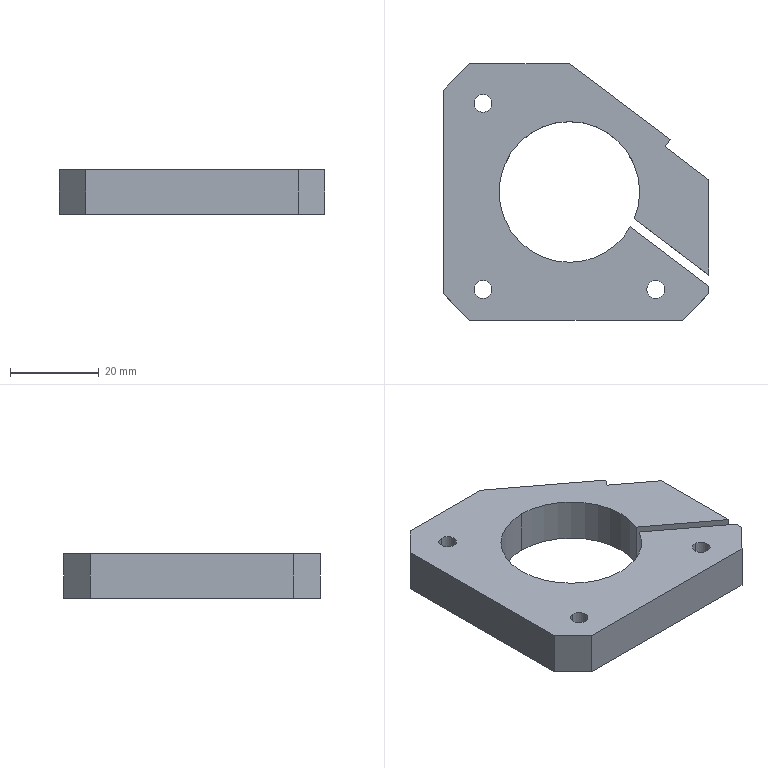Part | SolidWorks | features BaseBody 1 | 1 solid | 24 faces | box 60 x 58 x 10 mm | volume 21556 mm3 | plane 15 | cylinder 9 | commonest cylinder face diameters 4 x6 31.75 x3
STEP:
#1=CARTESIAN_POINT('',(17.98,-19.981,10.));
#2=VERTEX_POINT('',#1);
#3=CARTESIAN_POINT('',(17.98,-23.981,10.));
#4=VERTEX_POINT('',#3);
#5=CARTESIAN_POINT('',(17.98,-21.981,10.));
#6=DIRECTION('',(0.,0.,1.));
#7=DIRECTION('',(0.,1.,0.));
#8=AXIS2_PLACEMENT_3D('',#5,#6,#7);
#9=CIRCLE('',#8,2.);
#10=EDGE_CURVE('',#2,#4,#9,.T.);
#11=ORIENTED_EDGE('',*,*,#10,.T.);
#12=CARTESIAN_POINT('',(17.98,-23.981,0.));
#13=VERTEX_POINT('',#12);
#14=CARTESIAN_POINT('',(17.98,-23.981,10.));
#15=DIRECTION('',(0.,0.,-1.));
#16=VECTOR('',#15,1000.);
#17=LINE('',#14,#16);
#18=EDGE_CURVE('',#4,#13,#17,.T.);
#19=ORIENTED_EDGE('',*,*,#18,.T.);
#20=CARTESIAN_POINT('',(17.98,-19.981,0.));
#21=VERTEX_POINT('',#20);
#22=CARTESIAN_POINT('',(17.98,-21.981,0.));
#23=DIRECTION('',(0.,0.,-1.));
#24=DIRECTION('',(0.,1.,0.));
#25=AXIS2_PLACEMENT_3D('',#22,#23,#24);
#26=CIRCLE('',#25,2.);
#27=EDGE_CURVE('',#13,#21,#26,.T.);
#28=ORIENTED_EDGE('',*,*,#27,.T.);
#29=CARTESIAN_POINT('',(17.98,-19.981,10.));
#30=DIRECTION('',(0.,0.,-1.));
#31=VECTOR('',#30,1000.);
#32=LINE('',#29,#31);
#33=EDGE_CURVE('',#2,#21,#32,.T.);
#34=ORIENTED_EDGE('',*,*,#33,.F.);
#35=EDGE_LOOP('',(#11,#19,#28,#34));
#36=FACE_OUTER_BOUND('',#35,.T.);
#37=CARTESIAN_POINT('',(17.98,-21.981,10.));
#38=DIRECTION('',(0.,0.,-1.));
#39=DIRECTION('',(0.,1.,0.));
#40=AXIS2_PLACEMENT_3D('',#37,#38,#39);
#41=CYLINDRICAL_SURFACE('',#40,2.);
#42=ADVANCED_FACE('',(#36),#41,.F.);
#43=CARTESIAN_POINT('',(-21.02,18.019,10.));
#44=VERTEX_POINT('',#43);
#45=CARTESIAN_POINT('',(-21.02,22.019,10.));
#46=VERTEX_POINT('',#45);
#47=CARTESIAN_POINT('',(-21.02,20.019,10.));
#48=DIRECTION('',(0.,0.,-1.));
#49=DIRECTION('',(0.,1.,0.));
#50=AXIS2_PLACEMENT_3D('',#47,#48,#49);
#51=CIRCLE('',#50,2.);
#52=EDGE_CURVE('',#44,#46,#51,.T.);
#53=ORIENTED_EDGE('',*,*,#52,.F.);
#54=CARTESIAN_POINT('',(-21.02,18.019,0.));
#55=VERTEX_POINT('',#54);
#56=CARTESIAN_POINT('',(-21.02,18.019,10.));
#57=DIRECTION('',(0.,0.,-1.));
#58=VECTOR('',#57,1000.);
#59=LINE('',#56,#58);
#60=EDGE_CURVE('',#44,#55,#59,.T.);
#61=ORIENTED_EDGE('',*,*,#60,.T.);
#62=CARTESIAN_POINT('',(-21.02,22.019,0.));
#63=VERTEX_POINT('',#62);
#64=CARTESIAN_POINT('',(-21.02,20.019,0.));
#65=DIRECTION('',(0.,0.,-1.));
#66=DIRECTION('',(0.,1.,0.));
#67=AXIS2_PLACEMENT_3D('',#64,#65,#66);
#68=CIRCLE('',#67,2.);
#69=EDGE_CURVE('',#55,#63,#68,.T.);
#70=ORIENTED_EDGE('',*,*,#69,.T.);
#71=CARTESIAN_POINT('',(-21.02,22.019,10.));
#72=DIRECTION('',(0.,0.,-1.));
#73=VECTOR('',#72,1000.);
#74=LINE('',#71,#73);
#75=EDGE_CURVE('',#46,#63,#74,.T.);
#76=ORIENTED_EDGE('',*,*,#75,.F.);
#77=EDGE_LOOP('',(#53,#61,#70,#76));
#78=FACE_OUTER_BOUND('',#77,.T.);
#79=CARTESIAN_POINT('',(-21.02,20.019,10.));
#80=DIRECTION('',(0.,0.,-1.));
#81=DIRECTION('',(0.,1.,0.));
#82=AXIS2_PLACEMENT_3D('',#79,#80,#81);
#83=CYLINDRICAL_SURFACE('',#82,2.);
#84=ADVANCED_FACE('',(#78),#83,.F.);
#85=CARTESIAN_POINT('',(-21.02,-23.981,10.));
#86=VERTEX_POINT('',#85);
#87=CARTESIAN_POINT('',(-21.02,-19.981,10.));
#88=VERTEX_POINT('',#87);
#89=CARTESIAN_POINT('',(-21.02,-21.981,10.));
#90=DIRECTION('',(0.,0.,-1.));
#91=DIRECTION('',(0.,1.,0.));
#92=AXIS2_PLACEMENT_3D('',#89,#90,#91);
#93=CIRCLE('',#92,2.);
#94=EDGE_CURVE('',#86,#88,#93,.T.);
#95=ORIENTED_EDGE('',*,*,#94,.F.);
#96=CARTESIAN_POINT('',(-21.02,-23.981,0.));
#97=VERTEX_POINT('',#96);
#98=CARTESIAN_POINT('',(-21.02,-23.981,10.));
#99=DIRECTION('',(0.,0.,-1.));
#100=VECTOR('',#99,1000.);
#101=LINE('',#98,#100);
#102=EDGE_CURVE('',#86,#97,#101,.T.);
#103=ORIENTED_EDGE('',*,*,#102,.T.);
#104=CARTESIAN_POINT('',(-21.02,-19.981,0.));
#105=VERTEX_POINT('',#104);
#106=CARTESIAN_POINT('',(-21.02,-21.981,0.));
#107=DIRECTION('',(0.,0.,-1.));
#108=DIRECTION('',(0.,1.,0.));
#109=AXIS2_PLACEMENT_3D('',#106,#107,#108);
#110=CIRCLE('',#109,2.);
#111=EDGE_CURVE('',#97,#105,#110,.T.);
#112=ORIENTED_EDGE('',*,*,#111,.T.);
#113=CARTESIAN_POINT('',(-21.02,-19.981,10.));
#114=DIRECTION('',(0.,0.,-1.));
#115=VECTOR('',#114,1000.);
#116=LINE('',#113,#115);
#117=EDGE_CURVE('',#88,#105,#116,.T.);
#118=ORIENTED_EDGE('',*,*,#117,.F.);
#119=EDGE_LOOP('',(#95,#103,#112,#118));
#120=FACE_OUTER_BOUND('',#119,.T.);
#121=CARTESIAN_POINT('',(-21.02,-21.981,10.));
#122=DIRECTION('',(0.,0.,-1.));
#123=DIRECTION('',(0.,1.,0.));
#124=AXIS2_PLACEMENT_3D('',#121,#122,#123);
#125=CYLINDRICAL_SURFACE('',#124,2.);
#126=ADVANCED_FACE('',(#120),#125,.F.);
#127=CARTESIAN_POINT('',(-1.52,-15.856,10.));
#128=VERTEX_POINT('',#127);
#129=CARTESIAN_POINT('',(-1.52,15.894,10.));
#130=VERTEX_POINT('',#129);
#131=CARTESIAN_POINT('',(-1.52,0.01944,10.));
#132=DIRECTION('',(0.,0.,-1.));
#133=DIRECTION('',(0.,1.,0.));
#134=AXIS2_PLACEMENT_3D('',#131,#132,#133);
#135=CIRCLE('',#134,15.875);
#136=EDGE_CURVE('',#128,#130,#135,.T.);
#137=ORIENTED_EDGE('',*,*,#136,.F.);
#138=CARTESIAN_POINT('',(-1.52,-15.856,0.));
#139=VERTEX_POINT('',#138);
#140=CARTESIAN_POINT('',(-1.52,-15.856,10.));
#141=DIRECTION('',(0.,0.,-1.));
#142=VECTOR('',#141,1000.);
#143=LINE('',#140,#142);
#144=EDGE_CURVE('',#128,#139,#143,.T.);
#145=ORIENTED_EDGE('',*,*,#144,.T.);
#146=CARTESIAN_POINT('',(-1.52,15.894,0.));
#147=VERTEX_POINT('',#146);
#148=CARTESIAN_POINT('',(-1.52,0.01944,0.));
#149=DIRECTION('',(0.,0.,-1.));
#150=DIRECTION('',(0.,1.,0.));
#151=AXIS2_PLACEMENT_3D('',#148,#149,#150);
#152=CIRCLE('',#151,15.875);
#153=EDGE_CURVE('',#139,#147,#152,.T.);
#154=ORIENTED_EDGE('',*,*,#153,.T.);
#155=CARTESIAN_POINT('',(-1.52,15.894,10.));
#156=DIRECTION('',(0.,0.,-1.));
#157=VECTOR('',#156,1000.);
#158=LINE('',#155,#157);
#159=EDGE_CURVE('',#130,#147,#158,.T.);
#160=ORIENTED_EDGE('',*,*,#159,.F.);
#161=EDGE_LOOP('',(#137,#145,#154,#160));
#162=FACE_OUTER_BOUND('',#161,.T.);
#163=CARTESIAN_POINT('',(-1.52,0.01944,10.));
#164=DIRECTION('',(0.,0.,-1.));
#165=DIRECTION('',(0.,1.,0.));
#166=AXIS2_PLACEMENT_3D('',#163,#164,#165);
#167=CYLINDRICAL_SURFACE('',#166,15.875);
#168=ADVANCED_FACE('',(#162),#167,.F.);
#169=CARTESIAN_POINT('',(13.15,-6.048,10.));
#170=VERTEX_POINT('',#169);
#171=CARTESIAN_POINT('',(-1.52,0.01944,10.));
#172=DIRECTION('',(0.,0.,-1.));
#173=DIRECTION('',(0.,1.,0.));
#174=AXIS2_PLACEMENT_3D('',#171,#172,#173);
#175=CIRCLE('',#174,15.875);
#176=EDGE_CURVE('',#130,#170,#175,.T.);
#177=ORIENTED_EDGE('',*,*,#176,.F.);
#178=ORIENTED_EDGE('',*,*,#159,.T.);
#179=CARTESIAN_POINT('',(13.15,-6.048,0.));
#180=VERTEX_POINT('',#179);
#181=CARTESIAN_POINT('',(-1.52,0.01944,0.));
#182=DIRECTION('',(0.,0.,-1.));
#183=DIRECTION('',(0.,1.,0.));
#184=AXIS2_PLACEMENT_3D('',#181,#182,#183);
#185=CIRCLE('',#184,15.875);
#186=EDGE_CURVE('',#147,#180,#185,.T.);
#187=ORIENTED_EDGE('',*,*,#186,.T.);
#188=CARTESIAN_POINT('',(13.15,-6.048,5.));
#189=DIRECTION('',(0.,0.,1.));
#190=VECTOR('',#189,1000.);
#191=LINE('',#188,#190);
#192=EDGE_CURVE('',#180,#170,#191,.T.);
#193=ORIENTED_EDGE('',*,*,#192,.T.);
#194=EDGE_LOOP('',(#177,#178,#187,#193));
#195=FACE_OUTER_BOUND('',#194,.T.);
#196=CARTESIAN_POINT('',(-1.52,0.01944,10.));
#197=DIRECTION('',(0.,0.,-1.));
#198=DIRECTION('',(0.,1.,0.));
#199=AXIS2_PLACEMENT_3D('',#196,#197,#198);
#200=CYLINDRICAL_SURFACE('',#199,15.875);
#201=ADVANCED_FACE('',(#195),#200,.F.);
#202=ORIENTED_EDGE('',*,*,#18,.F.);
#203=CARTESIAN_POINT('',(17.98,-21.981,10.));
#204=DIRECTION('',(0.,0.,1.));
#205=DIRECTION('',(0.,1.,0.));
#206=AXIS2_PLACEMENT_3D('',#203,#204,#205);
#207=CIRCLE('',#206,2.);
#208=EDGE_CURVE('',#4,#2,#207,.T.);
#209=ORIENTED_EDGE('',*,*,#208,.T.);
#210=ORIENTED_EDGE('',*,*,#33,.T.);
#211=CARTESIAN_POINT('',(17.98,-21.981,0.));
#212=DIRECTION('',(0.,0.,-1.));
#213=DIRECTION('',(0.,1.,0.));
#214=AXIS2_PLACEMENT_3D('',#211,#212,#213);
#215=CIRCLE('',#214,2.);
#216=EDGE_CURVE('',#21,#13,#215,.T.);
#217=ORIENTED_EDGE('',*,*,#216,.T.);
#218=EDGE_LOOP('',(#202,#209,#210,#217));
#219=FACE_OUTER_BOUND('',#218,.T.);
#220=CARTESIAN_POINT('',(17.98,-21.981,10.));
#221=DIRECTION('',(0.,0.,-1.));
#222=DIRECTION('',(0.,1.,0.));
#223=AXIS2_PLACEMENT_3D('',#220,#221,#222);
#224=CYLINDRICAL_SURFACE('',#223,2.);
#225=ADVANCED_FACE('',(#219),#224,.F.);
#226=ORIENTED_EDGE('',*,*,#216,.F.);
#227=ORIENTED_EDGE('',*,*,#27,.F.);
#228=EDGE_LOOP('',(#226,#227));
#229=FACE_BOUND('',#228,.T.);
#230=CARTESIAN_POINT('',(-21.02,20.019,0.));
#231=DIRECTION('',(0.,0.,-1.));
#232=DIRECTION('',(0.,1.,0.));
#233=AXIS2_PLACEMENT_3D('',#230,#231,#232);
#234=CIRCLE('',#233,2.);
#235=EDGE_CURVE('',#63,#55,#234,.T.);
#236=ORIENTED_EDGE('',*,*,#235,.F.);
#237=ORIENTED_EDGE('',*,*,#69,.F.);
#238=EDGE_LOOP('',(#236,#237));
#239=FACE_BOUND('',#238,.T.);
#240=CARTESIAN_POINT('',(-21.02,-21.981,0.));
#241=DIRECTION('',(0.,0.,-1.));
#242=DIRECTION('',(0.,1.,0.));
#243=AXIS2_PLACEMENT_3D('',#240,#241,#242);
#244=CIRCLE('',#243,2.);
#245=EDGE_CURVE('',#105,#97,#244,.T.);
#246=ORIENTED_EDGE('',*,*,#245,.F.);
#247=ORIENTED_EDGE('',*,*,#111,.F.);
#248=EDGE_LOOP('',(#246,#247));
#249=FACE_BOUND('',#248,.T.);
#250=CARTESIAN_POINT('',(-30.02,-22.981,0.));
#251=VERTEX_POINT('',#250);
#252=CARTESIAN_POINT('',(-24.02,-28.981,0.));
#253=VERTEX_POINT('',#252);
#254=CARTESIAN_POINT('',(-24.02,-28.981,0.));
#255=DIRECTION('',(0.7071,-0.7071,0.));
#256=VECTOR('',#255,1000.);
#257=LINE('',#254,#256);
#258=EDGE_CURVE('',#251,#253,#257,.T.);
#259=ORIENTED_EDGE('',*,*,#258,.F.);
#260=CARTESIAN_POINT('',(-30.02,23.019,0.));
#261=VERTEX_POINT('',#260);
#262=CARTESIAN_POINT('',(-30.02,0.01944,0.));
#263=DIRECTION('',(0.,-1.,0.));
#264=VECTOR('',#263,1000.);
#265=LINE('',#262,#264);
#266=EDGE_CURVE('',#261,#251,#265,.T.);
#267=ORIENTED_EDGE('',*,*,#266,.F.);
#268=CARTESIAN_POINT('',(-24.02,29.019,0.));
#269=VERTEX_POINT('',#268);
#270=CARTESIAN_POINT('',(-30.02,23.019,0.));
#271=DIRECTION('',(-0.7071,-0.7071,0.));
#272=VECTOR('',#271,1000.);
#273=LINE('',#270,#272);
#274=EDGE_CURVE('',#269,#261,#273,.T.);
#275=ORIENTED_EDGE('',*,*,#274,.F.);
#276=CARTESIAN_POINT('',(-1.546,29.019,0.));
#277=VERTEX_POINT('',#276);
#278=CARTESIAN_POINT('',(-0.02011,29.019,0.));
#279=DIRECTION('',(-1.,0.,0.));
#280=VECTOR('',#279,1000.);
#281=LINE('',#278,#280);
#282=EDGE_CURVE('',#277,#269,#281,.T.);
#283=ORIENTED_EDGE('',*,*,#282,.F.);
#284=CARTESIAN_POINT('',(21.305,11.8,0.));
#285=VERTEX_POINT('',#284);
#286=CARTESIAN_POINT('',(-1.546,29.019,0.));
#287=DIRECTION('',(-0.7986,0.6018,0.));
#288=VECTOR('',#287,1000.);
#289=LINE('',#286,#288);
#290=EDGE_CURVE('',#285,#277,#289,.T.);
#291=ORIENTED_EDGE('',*,*,#290,.F.);
#292=CARTESIAN_POINT('',(20.101,10.203,0.));
#293=VERTEX_POINT('',#292);
#294=CARTESIAN_POINT('',(21.305,11.8,0.));
#295=DIRECTION('',(0.6018,0.7986,0.));
#296=VECTOR('',#295,1000.);
#297=LINE('',#294,#296);
#298=EDGE_CURVE('',#293,#285,#297,.T.);
#299=ORIENTED_EDGE('',*,*,#298,.F.);
#300=CARTESIAN_POINT('',(29.98,2.759,0.));
#301=VERTEX_POINT('',#300);
#302=CARTESIAN_POINT('',(20.101,10.203,0.));
#303=DIRECTION('',(-0.7986,0.6018,0.));
#304=VECTOR('',#303,1000.);
#305=LINE('',#302,#304);
#306=EDGE_CURVE('',#301,#293,#305,.T.);
#307=ORIENTED_EDGE('',*,*,#306,.F.);
#308=CARTESIAN_POINT('',(29.98,-18.73,0.));
#309=VERTEX_POINT('',#308);
#310=CARTESIAN_POINT('',(29.98,0.01944,0.));
#311=DIRECTION('',(0.,1.,0.));
#312=VECTOR('',#311,1000.);
#313=LINE('',#310,#312);
#314=EDGE_CURVE('',#309,#301,#313,.T.);
#315=ORIENTED_EDGE('',*,*,#314,.F.);
#316=CARTESIAN_POINT('',(29.98,-18.73,0.));
#317=DIRECTION('',(0.7986,-0.6018,0.));
#318=VECTOR('',#317,1000.);
#319=LINE('',#316,#318);
#320=EDGE_CURVE('',#180,#309,#319,.T.);
#321=ORIENTED_EDGE('',*,*,#320,.F.);
#322=ORIENTED_EDGE('',*,*,#186,.F.);
#323=ORIENTED_EDGE('',*,*,#153,.F.);
#324=CARTESIAN_POINT('',(12.252,-7.876,0.));
#325=VERTEX_POINT('',#324);
#326=CARTESIAN_POINT('',(-1.52,0.01944,0.));
#327=DIRECTION('',(0.,0.,-1.));
#328=DIRECTION('',(0.,1.,0.));
#329=AXIS2_PLACEMENT_3D('',#326,#327,#328);
#330=CIRCLE('',#329,15.875);
#331=EDGE_CURVE('',#325,#139,#330,.T.);
#332=ORIENTED_EDGE('',*,*,#331,.F.);
#333=CARTESIAN_POINT('',(29.98,-21.235,0.));
#334=VERTEX_POINT('',#333);
#335=CARTESIAN_POINT('',(12.252,-7.876,0.));
#336=DIRECTION('',(-0.7986,0.6018,0.));
#337=VECTOR('',#336,1000.);
#338=LINE('',#335,#337);
#339=EDGE_CURVE('',#334,#325,#338,.T.);
#340=ORIENTED_EDGE('',*,*,#339,.F.);
#341=CARTESIAN_POINT('',(29.98,-22.981,0.));
#342=VERTEX_POINT('',#341);
#343=CARTESIAN_POINT('',(29.98,0.01944,0.));
#344=DIRECTION('',(0.,1.,0.));
#345=VECTOR('',#344,1000.);
#346=LINE('',#343,#345);
#347=EDGE_CURVE('',#342,#334,#346,.T.);
#348=ORIENTED_EDGE('',*,*,#347,.F.);
#349=CARTESIAN_POINT('',(23.98,-28.981,0.));
#350=VERTEX_POINT('',#349);
#351=CARTESIAN_POINT('',(29.98,-22.981,0.));
#352=DIRECTION('',(0.7071,0.7071,0.));
#353=VECTOR('',#352,1000.);
#354=LINE('',#351,#353);
#355=EDGE_CURVE('',#350,#342,#354,.T.);
#356=ORIENTED_EDGE('',*,*,#355,.F.);
#357=CARTESIAN_POINT('',(-0.02011,-28.981,0.));
#358=DIRECTION('',(1.,0.,0.));
#359=VECTOR('',#358,1000.);
#360=LINE('',#357,#359);
#361=EDGE_CURVE('',#253,#350,#360,.T.);
#362=ORIENTED_EDGE('',*,*,#361,.F.);
#363=EDGE_LOOP('',(#259,#267,#275,#283,#291,#299,#307,#315,#321,#322,#323,#332,#340,#348,#356,#362));
#364=FACE_OUTER_BOUND('',#363,.T.);
#365=CARTESIAN_POINT('',(-30.02,-28.981,0.));
#366=DIRECTION('',(0.,0.,1.));
#367=DIRECTION('',(1.,0.,0.));
#368=AXIS2_PLACEMENT_3D('',#365,#366,#367);
#369=PLANE('',#368);
#370=ADVANCED_FACE('',(#229,#239,#249,#364),#369,.F.);
#371=ORIENTED_EDGE('',*,*,#10,.F.);
#372=ORIENTED_EDGE('',*,*,#208,.F.);
#373=EDGE_LOOP('',(#371,#372));
#374=FACE_BOUND('',#373,.T.);
#375=CARTESIAN_POINT('',(-21.02,20.019,10.));
#376=DIRECTION('',(0.,0.,-1.));
#377=DIRECTION('',(0.,1.,0.));
#378=AXIS2_PLACEMENT_3D('',#375,#376,#377);
#379=CIRCLE('',#378,2.);
#380=EDGE_CURVE('',#46,#44,#379,.T.);
#381=ORIENTED_EDGE('',*,*,#380,.T.);
#382=ORIENTED_EDGE('',*,*,#52,.T.);
#383=EDGE_LOOP('',(#381,#382));
#384=FACE_BOUND('',#383,.T.);
#385=CARTESIAN_POINT('',(-21.02,-21.981,10.));
#386=DIRECTION('',(0.,0.,-1.));
#387=DIRECTION('',(0.,1.,0.));
#388=AXIS2_PLACEMENT_3D('',#385,#386,#387);
#389=CIRCLE('',#388,2.);
#390=EDGE_CURVE('',#88,#86,#389,.T.);
#391=ORIENTED_EDGE('',*,*,#390,.T.);
#392=ORIENTED_EDGE('',*,*,#94,.T.);
#393=EDGE_LOOP('',(#391,#392));
#394=FACE_BOUND('',#393,.T.);
#395=CARTESIAN_POINT('',(-1.546,29.019,10.));
#396=VERTEX_POINT('',#395);
#397=CARTESIAN_POINT('',(-24.02,29.019,10.));
#398=VERTEX_POINT('',#397);
#399=CARTESIAN_POINT('',(-0.02011,29.019,10.));
#400=DIRECTION('',(-1.,0.,0.));
#401=VECTOR('',#400,1000.);
#402=LINE('',#399,#401);
#403=EDGE_CURVE('',#396,#398,#402,.T.);
#404=ORIENTED_EDGE('',*,*,#403,.T.);
#405=CARTESIAN_POINT('',(-30.02,23.019,10.));
#406=VERTEX_POINT('',#405);
#407=CARTESIAN_POINT('',(-24.02,29.019,10.));
#408=DIRECTION('',(-0.7071,-0.7071,0.));
#409=VECTOR('',#408,1000.);
#410=LINE('',#407,#409);
#411=EDGE_CURVE('',#398,#406,#410,.T.);
#412=ORIENTED_EDGE('',*,*,#411,.T.);
#413=CARTESIAN_POINT('',(-30.02,-22.981,10.));
#414=VERTEX_POINT('',#413);
#415=CARTESIAN_POINT('',(-30.02,0.01944,10.));
#416=DIRECTION('',(0.,-1.,0.));
#417=VECTOR('',#416,1000.);
#418=LINE('',#415,#417);
#419=EDGE_CURVE('',#406,#414,#418,.T.);
#420=ORIENTED_EDGE('',*,*,#419,.T.);
#421=CARTESIAN_POINT('',(-24.02,-28.981,10.));
#422=VERTEX_POINT('',#421);
#423=CARTESIAN_POINT('',(-30.02,-22.981,10.));
#424=DIRECTION('',(0.7071,-0.7071,0.));
#425=VECTOR('',#424,1000.);
#426=LINE('',#423,#425);
#427=EDGE_CURVE('',#414,#422,#426,.T.);
#428=ORIENTED_EDGE('',*,*,#427,.T.);
#429=CARTESIAN_POINT('',(23.98,-28.981,10.));
#430=VERTEX_POINT('',#429);
#431=CARTESIAN_POINT('',(-0.02011,-28.981,10.));
#432=DIRECTION('',(1.,0.,0.));
#433=VECTOR('',#432,1000.);
#434=LINE('',#431,#433);
#435=EDGE_CURVE('',#422,#430,#434,.T.);
#436=ORIENTED_EDGE('',*,*,#435,.T.);
#437=CARTESIAN_POINT('',(29.98,-22.981,10.));
#438=VERTEX_POINT('',#437);
#439=CARTESIAN_POINT('',(23.98,-28.981,10.));
#440=DIRECTION('',(0.7071,0.7071,0.));
#441=VECTOR('',#440,1000.);
#442=LINE('',#439,#441);
#443=EDGE_CURVE('',#430,#438,#442,.T.);
#444=ORIENTED_EDGE('',*,*,#443,.T.);
#445=CARTESIAN_POINT('',(29.98,-21.235,10.));
#446=VERTEX_POINT('',#445);
#447=CARTESIAN_POINT('',(29.98,0.01944,10.));
#448=DIRECTION('',(0.,1.,0.));
#449=VECTOR('',#448,1000.);
#450=LINE('',#447,#449);
#451=EDGE_CURVE('',#438,#446,#450,.T.);
#452=ORIENTED_EDGE('',*,*,#451,.T.);
#453=CARTESIAN_POINT('',(12.252,-7.876,10.));
#454=VERTEX_POINT('',#453);
#455=CARTESIAN_POINT('',(29.98,-21.235,10.));
#456=DIRECTION('',(-0.7986,0.6018,0.));
#457=VECTOR('',#456,1000.);
#458=LINE('',#455,#457);
#459=EDGE_CURVE('',#446,#454,#458,.T.);
#460=ORIENTED_EDGE('',*,*,#459,.T.);
#461=CARTESIAN_POINT('',(-1.52,0.01944,10.));
#462=DIRECTION('',(0.,0.,-1.));
#463=DIRECTION('',(0.,1.,0.));
#464=AXIS2_PLACEMENT_3D('',#461,#462,#463);
#465=CIRCLE('',#464,15.875);
#466=EDGE_CURVE('',#454,#128,#465,.T.);
#467=ORIENTED_EDGE('',*,*,#466,.T.);
#468=ORIENTED_EDGE('',*,*,#136,.T.);
#469=ORIENTED_EDGE('',*,*,#176,.T.);
#470=CARTESIAN_POINT('',(29.98,-18.73,10.));
#471=VERTEX_POINT('',#470);
#472=CARTESIAN_POINT('',(13.15,-6.048,10.));
#473=DIRECTION('',(0.7986,-0.6018,0.));
#474=VECTOR('',#473,1000.);
#475=LINE('',#472,#474);
#476=EDGE_CURVE('',#170,#471,#475,.T.);
#477=ORIENTED_EDGE('',*,*,#476,.T.);
#478=CARTESIAN_POINT('',(29.98,2.759,10.));
#479=VERTEX_POINT('',#478);
#480=CARTESIAN_POINT('',(29.98,0.01944,10.));
#481=DIRECTION('',(0.,1.,0.));
#482=VECTOR('',#481,1000.);
#483=LINE('',#480,#482);
#484=EDGE_CURVE('',#471,#479,#483,.T.);
#485=ORIENTED_EDGE('',*,*,#484,.T.);
#486=CARTESIAN_POINT('',(20.101,10.203,10.));
#487=VERTEX_POINT('',#486);
#488=CARTESIAN_POINT('',(29.98,2.759,10.));
#489=DIRECTION('',(-0.7986,0.6018,0.));
#490=VECTOR('',#489,1000.);
#491=LINE('',#488,#490);
#492=EDGE_CURVE('',#479,#487,#491,.T.);
#493=ORIENTED_EDGE('',*,*,#492,.T.);
#494=CARTESIAN_POINT('',(21.305,11.8,10.));
#495=VERTEX_POINT('',#494);
#496=CARTESIAN_POINT('',(20.101,10.203,10.));
#497=DIRECTION('',(0.6018,0.7986,0.));
#498=VECTOR('',#497,1000.);
#499=LINE('',#496,#498);
#500=EDGE_CURVE('',#487,#495,#499,.T.);
#501=ORIENTED_EDGE('',*,*,#500,.T.);
#502=CARTESIAN_POINT('',(21.305,11.8,10.));
#503=DIRECTION('',(-0.7986,0.6018,0.));
#504=VECTOR('',#503,1000.);
#505=LINE('',#502,#504);
#506=EDGE_CURVE('',#495,#396,#505,.T.);
#507=ORIENTED_EDGE('',*,*,#506,.T.);
#508=EDGE_LOOP('',(#404,#412,#420,#428,#436,#444,#452,#460,#467,#468,#469,#477,#485,#493,#501,#507));
#509=FACE_OUTER_BOUND('',#508,.T.);
#510=CARTESIAN_POINT('',(-30.02,-28.981,10.));
#511=DIRECTION('',(0.,0.,1.));
#512=DIRECTION('',(1.,0.,0.));
#513=AXIS2_PLACEMENT_3D('',#510,#511,#512);
#514=PLANE('',#513);
#515=ADVANCED_FACE('',(#374,#384,#394,#509),#514,.T.);
#516=ORIENTED_EDGE('',*,*,#60,.F.);
#517=ORIENTED_EDGE('',*,*,#380,.F.);
#518=ORIENTED_EDGE('',*,*,#75,.T.);
#519=ORIENTED_EDGE('',*,*,#235,.T.);
#520=EDGE_LOOP('',(#516,#517,#518,#519));
#521=FACE_OUTER_BOUND('',#520,.T.);
#522=CARTESIAN_POINT('',(-21.02,20.019,10.));
#523=DIRECTION('',(0.,0.,-1.));
#524=DIRECTION('',(0.,1.,0.));
#525=AXIS2_PLACEMENT_3D('',#522,#523,#524);
#526=CYLINDRICAL_SURFACE('',#525,2.);
#527=ADVANCED_FACE('',(#521),#526,.F.);
#528=ORIENTED_EDGE('',*,*,#102,.F.);
#529=ORIENTED_EDGE('',*,*,#390,.F.);
#530=ORIENTED_EDGE('',*,*,#117,.T.);
#531=ORIENTED_EDGE('',*,*,#245,.T.);
#532=EDGE_LOOP('',(#528,#529,#530,#531));
#533=FACE_OUTER_BOUND('',#532,.T.);
#534=CARTESIAN_POINT('',(-21.02,-21.981,10.));
#535=DIRECTION('',(0.,0.,-1.));
#536=DIRECTION('',(0.,1.,0.));
#537=AXIS2_PLACEMENT_3D('',#534,#535,#536);
#538=CYLINDRICAL_SURFACE('',#537,2.);
#539=ADVANCED_FACE('',(#533),#538,.F.);
#540=CARTESIAN_POINT('',(-24.02,-28.981,5.));
#541=DIRECTION('',(0.,0.,1.));
#542=VECTOR('',#541,1000.);
#543=LINE('',#540,#542);
#544=EDGE_CURVE('',#253,#422,#543,.T.);
#545=ORIENTED_EDGE('',*,*,#544,.F.);
#546=ORIENTED_EDGE('',*,*,#361,.T.);
#547=CARTESIAN_POINT('',(23.98,-28.981,5.));
#548=DIRECTION('',(0.,0.,-1.));
#549=VECTOR('',#548,1000.);
#550=LINE('',#547,#549);
#551=EDGE_CURVE('',#430,#350,#550,.T.);
#552=ORIENTED_EDGE('',*,*,#551,.F.);
#553=ORIENTED_EDGE('',*,*,#435,.F.);
#554=EDGE_LOOP('',(#545,#546,#552,#553));
#555=FACE_OUTER_BOUND('',#554,.T.);
#556=CARTESIAN_POINT('',(23.98,-28.981,0.));
#557=DIRECTION('',(0.,1.,0.));
#558=DIRECTION('',(-1.,0.,0.));
#559=AXIS2_PLACEMENT_3D('',#556,#557,#558);
#560=PLANE('',#559);
#561=ADVANCED_FACE('',(#555),#560,.F.);
#562=CARTESIAN_POINT('',(-30.02,-22.981,5.));
#563=DIRECTION('',(0.,0.,1.));
#564=VECTOR('',#563,1000.);
#565=LINE('',#562,#564);
#566=EDGE_CURVE('',#251,#414,#565,.T.);
#567=ORIENTED_EDGE('',*,*,#566,.F.);
#568=ORIENTED_EDGE('',*,*,#258,.T.);
#569=ORIENTED_EDGE('',*,*,#544,.T.);
#570=ORIENTED_EDGE('',*,*,#427,.F.);
#571=EDGE_LOOP('',(#567,#568,#569,#570));
#572=FACE_OUTER_BOUND('',#571,.T.);
#573=CARTESIAN_POINT('',(-24.02,-28.981,0.));
#574=DIRECTION('',(0.7071,0.7071,0.));
#575=DIRECTION('',(-0.7071,0.7071,0.));
#576=AXIS2_PLACEMENT_3D('',#573,#574,#575);
#577=PLANE('',#576);
#578=ADVANCED_FACE('',(#572),#577,.F.);
#579=ORIENTED_EDGE('',*,*,#566,.T.);
#580=ORIENTED_EDGE('',*,*,#419,.F.);
#581=CARTESIAN_POINT('',(-30.02,23.019,5.));
#582=DIRECTION('',(0.,0.,1.));
#583=VECTOR('',#582,1000.);
#584=LINE('',#581,#583);
#585=EDGE_CURVE('',#261,#406,#584,.T.);
#586=ORIENTED_EDGE('',*,*,#585,.F.);
#587=ORIENTED_EDGE('',*,*,#266,.T.);
#588=EDGE_LOOP('',(#579,#580,#586,#587));
#589=FACE_OUTER_BOUND('',#588,.T.);
#590=CARTESIAN_POINT('',(-30.02,-22.981,0.));
#591=DIRECTION('',(1.,0.,0.));
#592=DIRECTION('',(0.,1.,0.));
#593=AXIS2_PLACEMENT_3D('',#590,#591,#592);
#594=PLANE('',#593);
#595=ADVANCED_FACE('',(#589),#594,.F.);
#596=CARTESIAN_POINT('',(-24.02,29.019,5.));
#597=DIRECTION('',(0.,0.,1.));
#598=VECTOR('',#597,1000.);
#599=LINE('',#596,#598);
#600=EDGE_CURVE('',#269,#398,#599,.T.);
#601=ORIENTED_EDGE('',*,*,#600,.F.);
#602=ORIENTED_EDGE('',*,*,#274,.T.);
#603=ORIENTED_EDGE('',*,*,#585,.T.);
#604=ORIENTED_EDGE('',*,*,#411,.F.);
#605=EDGE_LOOP('',(#601,#602,#603,#604));
#606=FACE_OUTER_BOUND('',#605,.T.);
#607=CARTESIAN_POINT('',(-30.02,23.019,0.));
#608=DIRECTION('',(0.7071,-0.7071,0.));
#609=DIRECTION('',(0.7071,0.7071,0.));
#610=AXIS2_PLACEMENT_3D('',#607,#608,#609);
#611=PLANE('',#610);
#612=ADVANCED_FACE('',(#606),#611,.F.);
#613=ORIENTED_EDGE('',*,*,#600,.T.);
#614=ORIENTED_EDGE('',*,*,#403,.F.);
#615=CARTESIAN_POINT('',(-1.546,29.019,5.));
#616=DIRECTION('',(0.,0.,1.));
#617=VECTOR('',#616,1000.);
#618=LINE('',#615,#617);
#619=EDGE_CURVE('',#277,#396,#618,.T.);
#620=ORIENTED_EDGE('',*,*,#619,.F.);
#621=ORIENTED_EDGE('',*,*,#282,.T.);
#622=EDGE_LOOP('',(#613,#614,#620,#621));
#623=FACE_OUTER_BOUND('',#622,.T.);
#624=CARTESIAN_POINT('',(-24.02,29.019,0.));
#625=DIRECTION('',(0.,-1.,0.));
#626=DIRECTION('',(1.,0.,0.));
#627=AXIS2_PLACEMENT_3D('',#624,#625,#626);
#628=PLANE('',#627);
#629=ADVANCED_FACE('',(#623),#628,.F.);
#630=ORIENTED_EDGE('',*,*,#619,.T.);
#631=ORIENTED_EDGE('',*,*,#506,.F.);
#632=CARTESIAN_POINT('',(21.305,11.8,5.));
#633=DIRECTION('',(0.,0.,1.));
#634=VECTOR('',#633,1000.);
#635=LINE('',#632,#634);
#636=EDGE_CURVE('',#285,#495,#635,.T.);
#637=ORIENTED_EDGE('',*,*,#636,.F.);
#638=ORIENTED_EDGE('',*,*,#290,.T.);
#639=EDGE_LOOP('',(#630,#631,#637,#638));
#640=FACE_OUTER_BOUND('',#639,.T.);
#641=CARTESIAN_POINT('',(-1.546,29.019,0.));
#642=DIRECTION('',(-0.6018,-0.7986,0.));
#643=DIRECTION('',(0.7986,-0.6018,0.));
#644=AXIS2_PLACEMENT_3D('',#641,#642,#643);
#645=PLANE('',#644);
#646=ADVANCED_FACE('',(#640),#645,.F.);
#647=ORIENTED_EDGE('',*,*,#636,.T.);
#648=ORIENTED_EDGE('',*,*,#500,.F.);
#649=CARTESIAN_POINT('',(20.101,10.203,5.));
#650=DIRECTION('',(0.,0.,1.));
#651=VECTOR('',#650,1000.);
#652=LINE('',#649,#651);
#653=EDGE_CURVE('',#293,#487,#652,.T.);
#654=ORIENTED_EDGE('',*,*,#653,.F.);
#655=ORIENTED_EDGE('',*,*,#298,.T.);
#656=EDGE_LOOP('',(#647,#648,#654,#655));
#657=FACE_OUTER_BOUND('',#656,.T.);
#658=CARTESIAN_POINT('',(21.305,11.8,0.));
#659=DIRECTION('',(-0.7986,0.6018,0.));
#660=DIRECTION('',(-0.6018,-0.7986,0.));
#661=AXIS2_PLACEMENT_3D('',#658,#659,#660);
#662=PLANE('',#661);
#663=ADVANCED_FACE('',(#657),#662,.F.);
#664=ORIENTED_EDGE('',*,*,#653,.T.);
#665=ORIENTED_EDGE('',*,*,#492,.F.);
#666=CARTESIAN_POINT('',(29.98,2.759,5.));
#667=DIRECTION('',(0.,0.,1.));
#668=VECTOR('',#667,1000.);
#669=LINE('',#666,#668);
#670=EDGE_CURVE('',#301,#479,#669,.T.);
#671=ORIENTED_EDGE('',*,*,#670,.F.);
#672=ORIENTED_EDGE('',*,*,#306,.T.);
#673=EDGE_LOOP('',(#664,#665,#671,#672));
#674=FACE_OUTER_BOUND('',#673,.T.);
#675=CARTESIAN_POINT('',(20.101,10.203,0.));
#676=DIRECTION('',(-0.6018,-0.7986,0.));
#677=DIRECTION('',(0.7986,-0.6018,0.));
#678=AXIS2_PLACEMENT_3D('',#675,#676,#677);
#679=PLANE('',#678);
#680=ADVANCED_FACE('',(#674),#679,.F.);
#681=ORIENTED_EDGE('',*,*,#670,.T.);
#682=ORIENTED_EDGE('',*,*,#484,.F.);
#683=CARTESIAN_POINT('',(29.98,-18.73,5.));
#684=DIRECTION('',(0.,0.,1.));
#685=VECTOR('',#684,1000.);
#686=LINE('',#683,#685);
#687=EDGE_CURVE('',#309,#471,#686,.T.);
#688=ORIENTED_EDGE('',*,*,#687,.F.);
#689=ORIENTED_EDGE('',*,*,#314,.T.);
#690=EDGE_LOOP('',(#681,#682,#688,#689));
#691=FACE_OUTER_BOUND('',#690,.T.);
#692=CARTESIAN_POINT('',(29.98,2.759,0.));
#693=DIRECTION('',(-1.,0.,0.));
#694=DIRECTION('',(0.,-1.,0.));
#695=AXIS2_PLACEMENT_3D('',#692,#693,#694);
#696=PLANE('',#695);
#697=ADVANCED_FACE('',(#691),#696,.F.);
#698=ORIENTED_EDGE('',*,*,#687,.T.);
#699=ORIENTED_EDGE('',*,*,#476,.F.);
#700=ORIENTED_EDGE('',*,*,#192,.F.);
#701=ORIENTED_EDGE('',*,*,#320,.T.);
#702=EDGE_LOOP('',(#698,#699,#700,#701));
#703=FACE_OUTER_BOUND('',#702,.T.);
#704=CARTESIAN_POINT('',(29.98,-18.73,0.));
#705=DIRECTION('',(0.6018,0.7986,0.));
#706=DIRECTION('',(-0.7986,0.6018,0.));
#707=AXIS2_PLACEMENT_3D('',#704,#705,#706);
#708=PLANE('',#707);
#709=ADVANCED_FACE('',(#703),#708,.F.);
#710=ORIENTED_EDGE('',*,*,#144,.F.);
#711=ORIENTED_EDGE('',*,*,#466,.F.);
#712=CARTESIAN_POINT('',(12.252,-7.876,5.));
#713=DIRECTION('',(0.,0.,-1.));
#714=VECTOR('',#713,1000.);
#715=LINE('',#712,#714);
#716=EDGE_CURVE('',#454,#325,#715,.T.);
#717=ORIENTED_EDGE('',*,*,#716,.T.);
#718=ORIENTED_EDGE('',*,*,#331,.T.);
#719=EDGE_LOOP('',(#710,#711,#717,#718));
#720=FACE_OUTER_BOUND('',#719,.T.);
#721=CARTESIAN_POINT('',(-1.52,0.01944,10.));
#722=DIRECTION('',(0.,0.,-1.));
#723=DIRECTION('',(0.,1.,0.));
#724=AXIS2_PLACEMENT_3D('',#721,#722,#723);
#725=CYLINDRICAL_SURFACE('',#724,15.875);
#726=ADVANCED_FACE('',(#720),#725,.F.);
#727=ORIENTED_EDGE('',*,*,#716,.F.);
#728=ORIENTED_EDGE('',*,*,#459,.F.);
#729=CARTESIAN_POINT('',(29.98,-21.235,5.));
#730=DIRECTION('',(0.,0.,1.));
#731=VECTOR('',#730,1000.);
#732=LINE('',#729,#731);
#733=EDGE_CURVE('',#334,#446,#732,.T.);
#734=ORIENTED_EDGE('',*,*,#733,.F.);
#735=ORIENTED_EDGE('',*,*,#339,.T.);
#736=EDGE_LOOP('',(#727,#728,#734,#735));
#737=FACE_OUTER_BOUND('',#736,.T.);
#738=CARTESIAN_POINT('',(12.252,-7.876,0.));
#739=DIRECTION('',(-0.6018,-0.7986,0.));
#740=DIRECTION('',(0.7986,-0.6018,0.));
#741=AXIS2_PLACEMENT_3D('',#738,#739,#740);
#742=PLANE('',#741);
#743=ADVANCED_FACE('',(#737),#742,.F.);
#744=CARTESIAN_POINT('',(29.98,-22.981,5.));
#745=DIRECTION('',(0.,0.,1.));
#746=VECTOR('',#745,1000.);
#747=LINE('',#744,#746);
#748=EDGE_CURVE('',#342,#438,#747,.T.);
#749=ORIENTED_EDGE('',*,*,#748,.F.);
#750=ORIENTED_EDGE('',*,*,#347,.T.);
#751=ORIENTED_EDGE('',*,*,#733,.T.);
#752=ORIENTED_EDGE('',*,*,#451,.F.);
#753=EDGE_LOOP('',(#749,#750,#751,#752));
#754=FACE_OUTER_BOUND('',#753,.T.);
#755=CARTESIAN_POINT('',(29.98,-22.981,0.));
#756=DIRECTION('',(-1.,0.,0.));
#757=DIRECTION('',(0.,0.,1.));
#758=AXIS2_PLACEMENT_3D('',#755,#756,#757);
#759=PLANE('',#758);
#760=ADVANCED_FACE('',(#754),#759,.F.);
#761=ORIENTED_EDGE('',*,*,#551,.T.);
#762=ORIENTED_EDGE('',*,*,#355,.T.);
#763=ORIENTED_EDGE('',*,*,#748,.T.);
#764=ORIENTED_EDGE('',*,*,#443,.F.);
#765=EDGE_LOOP('',(#761,#762,#763,#764));
#766=FACE_OUTER_BOUND('',#765,.T.);
#767=CARTESIAN_POINT('',(29.98,-22.981,0.));
#768=DIRECTION('',(-0.7071,0.7071,0.));
#769=DIRECTION('',(-0.7071,-0.7071,0.));
#770=AXIS2_PLACEMENT_3D('',#767,#768,#769);
#771=PLANE('',#770);
#772=ADVANCED_FACE('',(#766),#771,.F.);
#773=CLOSED_SHELL('',(#42,#84,#126,#168,#201,#225,#370,#515,#527,#539,#561,#578,#595,#612,#629,#646,#663,#680,#697,#709,#726,#743,#760,#772));
#774=MANIFOLD_SOLID_BREP('',#773);
#775=CARTESIAN_POINT('',(0.,0.,0.));
#776=DIRECTION('',(0.,0.,1.));
#777=DIRECTION('',(1.,0.,0.));
#778=AXIS2_PLACEMENT_3D('',#775,#776,#777);
#779=(LENGTH_UNIT()NAMED_UNIT(*)SI_UNIT(.MILLI.,.METRE.));
#780=UNCERTAINTY_MEASURE_WITH_UNIT(LENGTH_MEASURE(0.00001),#779,'','');
#781=(NAMED_UNIT(*)PLANE_ANGLE_UNIT()SI_UNIT($,.RADIAN.));
#782=(NAMED_UNIT(*)SI_UNIT($,.STERADIAN.)SOLID_ANGLE_UNIT());
#783=(GEOMETRIC_REPRESENTATION_CONTEXT(3)GLOBAL_UNCERTAINTY_ASSIGNED_CONTEXT((#780))GLOBAL_UNIT_ASSIGNED_CONTEXT((#779,#781,#782))REPRESENTATION_CONTEXT('',''));
#784=ADVANCED_BREP_SHAPE_REPRESENTATION('',(#774,#778),#783);